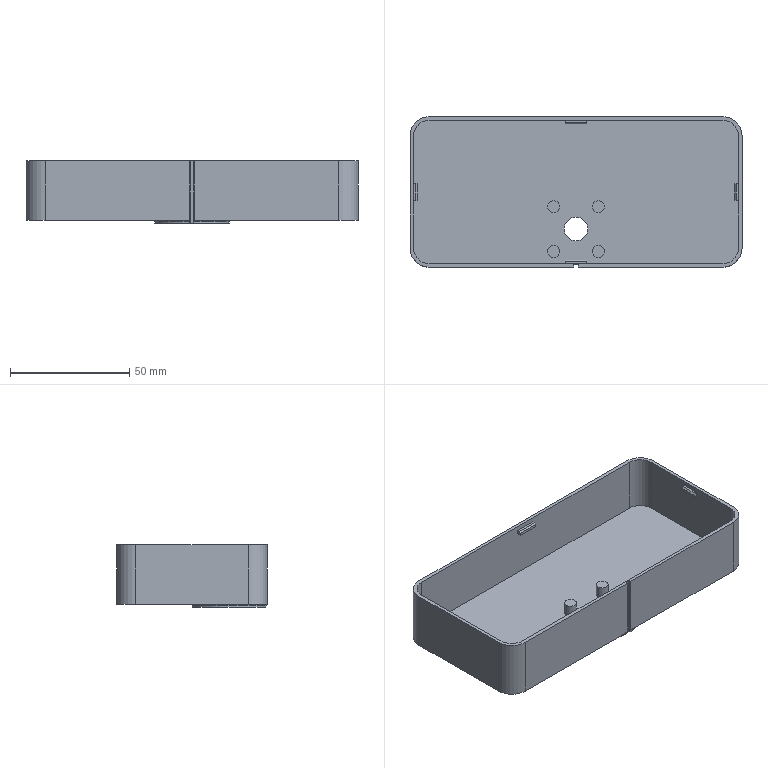Part | SolidWorks | features ICE 11, Fillet 4, Chamfer 2, MirrorPattern 2, Extrusion 1, Shell 1 | 1 solid | 105 faces | box 139 x 63 x 26.2 mm | volume 27399 mm3 | plane 55 | cylinder 39 | torus 11 | commonest cylinder face diameters 1 x8 5 x8 16 x6 13 x4 31 x3 0.4 x2